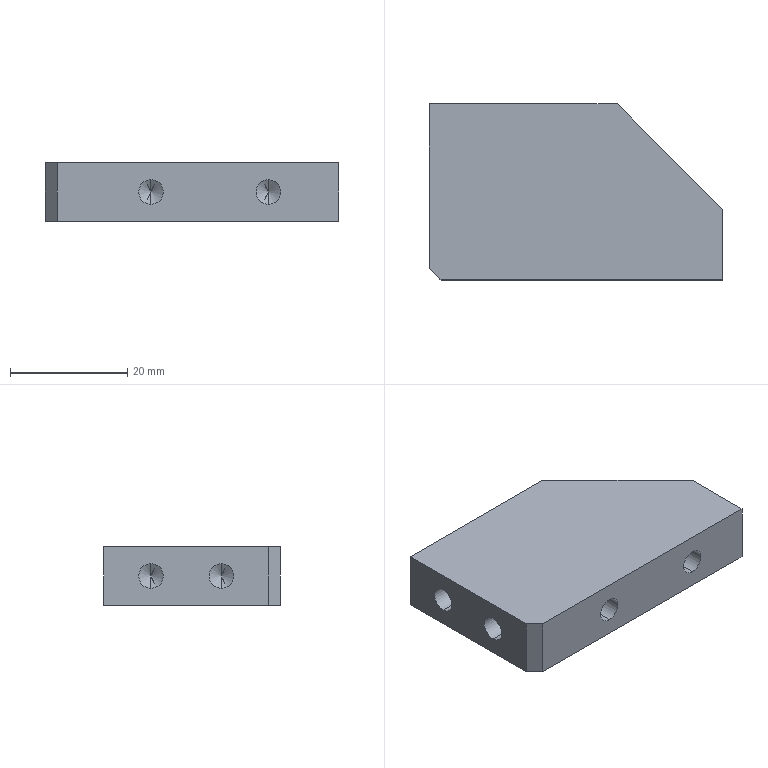Part | SolidWorks | features HoleWzd 2, Chamfer 1, Extrusion 1 | 1 solid | 24 faces | box 50 x 30 x 10 mm | volume 12561 mm3 | cylinder 8 | cone 8 | plane 8 | commonest cylinder face diameters 4.2 x8
STEP:
#1=CARTESIAN_POINT('',(30.,-6.912,7.1));
#2=VERTEX_POINT('',#1);
#3=CARTESIAN_POINT('',(30.,-6.912,2.9));
#4=VERTEX_POINT('',#3);
#5=CARTESIAN_POINT('',(30.,-6.912,5.));
#6=DIRECTION('',(0.,-1.,0.));
#7=DIRECTION('',(0.,0.,-1.));
#8=AXIS2_PLACEMENT_3D('',#5,#6,#7);
#9=CIRCLE('',#8,2.1);
#10=EDGE_CURVE('',#2,#4,#9,.T.);
#11=ORIENTED_EDGE('',*,*,#10,.F.);
#12=CARTESIAN_POINT('',(30.,-20.912,7.1));
#13=VERTEX_POINT('',#12);
#14=CARTESIAN_POINT('',(30.,-20.912,7.1));
#15=DIRECTION('',(0.,-1.,0.));
#16=VECTOR('',#15,1000.);
#17=LINE('',#14,#16);
#18=EDGE_CURVE('',#2,#13,#17,.T.);
#19=ORIENTED_EDGE('',*,*,#18,.T.);
#20=CARTESIAN_POINT('',(30.,-20.912,2.9));
#21=VERTEX_POINT('',#20);
#22=CARTESIAN_POINT('',(30.,-20.912,5.));
#23=DIRECTION('',(0.,-1.,0.));
#24=DIRECTION('',(0.,0.,-1.));
#25=AXIS2_PLACEMENT_3D('',#22,#23,#24);
#26=CIRCLE('',#25,2.1);
#27=EDGE_CURVE('',#13,#21,#26,.T.);
#28=ORIENTED_EDGE('',*,*,#27,.T.);
#29=CARTESIAN_POINT('',(30.,-20.912,2.9));
#30=DIRECTION('',(0.,-1.,0.));
#31=VECTOR('',#30,1000.);
#32=LINE('',#29,#31);
#33=EDGE_CURVE('',#4,#21,#32,.T.);
#34=ORIENTED_EDGE('',*,*,#33,.F.);
#35=EDGE_LOOP('',(#11,#19,#28,#34));
#36=FACE_OUTER_BOUND('',#35,.T.);
#37=CARTESIAN_POINT('',(30.,-20.912,5.));
#38=DIRECTION('',(0.,-1.,0.));
#39=DIRECTION('',(0.,0.,-1.));
#40=AXIS2_PLACEMENT_3D('',#37,#38,#39);
#41=CYLINDRICAL_SURFACE('',#40,2.1);
#42=ADVANCED_FACE('',(#36),#41,.F.);
#43=CARTESIAN_POINT('',(30.,-5.65,5.));
#44=VERTEX_POINT('',#43);
#45=CARTESIAN_POINT('',(30.,-6.912,2.9));
#46=DIRECTION('',(0.,-0.515,-0.8572));
#47=VECTOR('',#46,1000.);
#48=LINE('',#45,#47);
#49=EDGE_CURVE('',#44,#4,#48,.T.);
#50=ORIENTED_EDGE('',*,*,#49,.F.);
#51=CARTESIAN_POINT('',(30.,-6.912,7.1));
#52=DIRECTION('',(0.,-0.515,0.8572));
#53=VECTOR('',#52,1000.);
#54=LINE('',#51,#53);
#55=EDGE_CURVE('',#44,#2,#54,.T.);
#56=ORIENTED_EDGE('',*,*,#55,.T.);
#57=ORIENTED_EDGE('',*,*,#10,.T.);
#58=EDGE_LOOP('',(#50,#56,#57));
#59=FACE_OUTER_BOUND('',#58,.T.);
#60=CARTESIAN_POINT('',(30.,-6.912,5.));
#61=DIRECTION('',(0.,-1.,0.));
#62=DIRECTION('',(0.,0.,-1.));
#63=AXIS2_PLACEMENT_3D('',#60,#61,#62);
#64=CONICAL_SURFACE('',#63,2.1,1.03);
#65=ADVANCED_FACE('',(#59),#64,.F.);
#66=CARTESIAN_POINT('',(50.,-6.912,7.1));
#67=VERTEX_POINT('',#66);
#68=CARTESIAN_POINT('',(50.,-6.912,2.9));
#69=VERTEX_POINT('',#68);
#70=CARTESIAN_POINT('',(50.,-6.912,5.));
#71=DIRECTION('',(0.,-1.,0.));
#72=DIRECTION('',(0.,0.,-1.));
#73=AXIS2_PLACEMENT_3D('',#70,#71,#72);
#74=CIRCLE('',#73,2.1);
#75=EDGE_CURVE('',#67,#69,#74,.T.);
#76=ORIENTED_EDGE('',*,*,#75,.F.);
#77=CARTESIAN_POINT('',(50.,-20.912,7.1));
#78=VERTEX_POINT('',#77);
#79=CARTESIAN_POINT('',(50.,-20.912,7.1));
#80=DIRECTION('',(0.,-1.,0.));
#81=VECTOR('',#80,1000.);
#82=LINE('',#79,#81);
#83=EDGE_CURVE('',#67,#78,#82,.T.);
#84=ORIENTED_EDGE('',*,*,#83,.T.);
#85=CARTESIAN_POINT('',(50.,-20.912,2.9));
#86=VERTEX_POINT('',#85);
#87=CARTESIAN_POINT('',(50.,-20.912,5.));
#88=DIRECTION('',(0.,-1.,0.));
#89=DIRECTION('',(0.,0.,-1.));
#90=AXIS2_PLACEMENT_3D('',#87,#88,#89);
#91=CIRCLE('',#90,2.1);
#92=EDGE_CURVE('',#78,#86,#91,.T.);
#93=ORIENTED_EDGE('',*,*,#92,.T.);
#94=CARTESIAN_POINT('',(50.,-20.912,2.9));
#95=DIRECTION('',(0.,-1.,0.));
#96=VECTOR('',#95,1000.);
#97=LINE('',#94,#96);
#98=EDGE_CURVE('',#69,#86,#97,.T.);
#99=ORIENTED_EDGE('',*,*,#98,.F.);
#100=EDGE_LOOP('',(#76,#84,#93,#99));
#101=FACE_OUTER_BOUND('',#100,.T.);
#102=CARTESIAN_POINT('',(50.,-20.912,5.));
#103=DIRECTION('',(0.,-1.,0.));
#104=DIRECTION('',(0.,0.,-1.));
#105=AXIS2_PLACEMENT_3D('',#102,#103,#104);
#106=CYLINDRICAL_SURFACE('',#105,2.1);
#107=ADVANCED_FACE('',(#101),#106,.F.);
#108=CARTESIAN_POINT('',(50.,-5.65,5.));
#109=VERTEX_POINT('',#108);
#110=CARTESIAN_POINT('',(50.,-6.912,2.9));
#111=DIRECTION('',(0.,-0.515,-0.8572));
#112=VECTOR('',#111,1000.);
#113=LINE('',#110,#112);
#114=EDGE_CURVE('',#109,#69,#113,.T.);
#115=ORIENTED_EDGE('',*,*,#114,.F.);
#116=CARTESIAN_POINT('',(50.,-6.912,7.1));
#117=DIRECTION('',(0.,-0.515,0.8572));
#118=VECTOR('',#117,1000.);
#119=LINE('',#116,#118);
#120=EDGE_CURVE('',#109,#67,#119,.T.);
#121=ORIENTED_EDGE('',*,*,#120,.T.);
#122=ORIENTED_EDGE('',*,*,#75,.T.);
#123=EDGE_LOOP('',(#115,#121,#122));
#124=FACE_OUTER_BOUND('',#123,.T.);
#125=CARTESIAN_POINT('',(50.,-6.912,5.));
#126=DIRECTION('',(0.,-1.,0.));
#127=DIRECTION('',(0.,0.,-1.));
#128=AXIS2_PLACEMENT_3D('',#125,#126,#127);
#129=CONICAL_SURFACE('',#128,2.1,1.03);
#130=ADVANCED_FACE('',(#124),#129,.F.);
#131=CARTESIAN_POINT('',(26.,-10.912,2.9));
#132=VERTEX_POINT('',#131);
#133=CARTESIAN_POINT('',(26.,-10.912,7.1));
#134=VERTEX_POINT('',#133);
#135=CARTESIAN_POINT('',(26.,-10.912,5.));
#136=DIRECTION('',(-1.,0.,0.));
#137=DIRECTION('',(0.,0.,1.));
#138=AXIS2_PLACEMENT_3D('',#135,#136,#137);
#139=CIRCLE('',#138,2.1);
#140=EDGE_CURVE('',#132,#134,#139,.T.);
#141=ORIENTED_EDGE('',*,*,#140,.F.);
#142=CARTESIAN_POINT('',(12.,-10.912,2.9));
#143=VERTEX_POINT('',#142);
#144=CARTESIAN_POINT('',(12.,-10.912,2.9));
#145=DIRECTION('',(-1.,0.,0.));
#146=VECTOR('',#145,1000.);
#147=LINE('',#144,#146);
#148=EDGE_CURVE('',#132,#143,#147,.T.);
#149=ORIENTED_EDGE('',*,*,#148,.T.);
#150=CARTESIAN_POINT('',(12.,-10.912,7.1));
#151=VERTEX_POINT('',#150);
#152=CARTESIAN_POINT('',(12.,-10.912,5.));
#153=DIRECTION('',(-1.,0.,0.));
#154=DIRECTION('',(0.,0.,1.));
#155=AXIS2_PLACEMENT_3D('',#152,#153,#154);
#156=CIRCLE('',#155,2.1);
#157=EDGE_CURVE('',#143,#151,#156,.T.);
#158=ORIENTED_EDGE('',*,*,#157,.T.);
#159=CARTESIAN_POINT('',(12.,-10.912,7.1));
#160=DIRECTION('',(-1.,0.,0.));
#161=VECTOR('',#160,1000.);
#162=LINE('',#159,#161);
#163=EDGE_CURVE('',#134,#151,#162,.T.);
#164=ORIENTED_EDGE('',*,*,#163,.F.);
#165=EDGE_LOOP('',(#141,#149,#158,#164));
#166=FACE_OUTER_BOUND('',#165,.T.);
#167=CARTESIAN_POINT('',(12.,-10.912,5.));
#168=DIRECTION('',(-1.,0.,0.));
#169=DIRECTION('',(0.,0.,1.));
#170=AXIS2_PLACEMENT_3D('',#167,#168,#169);
#171=CYLINDRICAL_SURFACE('',#170,2.1);
#172=ADVANCED_FACE('',(#166),#171,.F.);
#173=CARTESIAN_POINT('',(27.262,-10.912,5.));
#174=VERTEX_POINT('',#173);
#175=CARTESIAN_POINT('',(26.,-10.912,7.1));
#176=DIRECTION('',(-0.515,0.,0.8572));
#177=VECTOR('',#176,1000.);
#178=LINE('',#175,#177);
#179=EDGE_CURVE('',#174,#134,#178,.T.);
#180=ORIENTED_EDGE('',*,*,#179,.F.);
#181=CARTESIAN_POINT('',(26.,-10.912,2.9));
#182=DIRECTION('',(-0.515,0.,-0.8572));
#183=VECTOR('',#182,1000.);
#184=LINE('',#181,#183);
#185=EDGE_CURVE('',#174,#132,#184,.T.);
#186=ORIENTED_EDGE('',*,*,#185,.T.);
#187=ORIENTED_EDGE('',*,*,#140,.T.);
#188=EDGE_LOOP('',(#180,#186,#187));
#189=FACE_OUTER_BOUND('',#188,.T.);
#190=CARTESIAN_POINT('',(26.,-10.912,5.));
#191=DIRECTION('',(-1.,0.,0.));
#192=DIRECTION('',(0.,0.,1.));
#193=AXIS2_PLACEMENT_3D('',#190,#191,#192);
#194=CONICAL_SURFACE('',#193,2.1,1.03);
#195=ADVANCED_FACE('',(#189),#194,.F.);
#196=CARTESIAN_POINT('',(26.,1.088,2.9));
#197=VERTEX_POINT('',#196);
#198=CARTESIAN_POINT('',(26.,1.088,7.1));
#199=VERTEX_POINT('',#198);
#200=CARTESIAN_POINT('',(26.,1.088,5.));
#201=DIRECTION('',(-1.,0.,0.));
#202=DIRECTION('',(0.,0.,1.));
#203=AXIS2_PLACEMENT_3D('',#200,#201,#202);
#204=CIRCLE('',#203,2.1);
#205=EDGE_CURVE('',#197,#199,#204,.T.);
#206=ORIENTED_EDGE('',*,*,#205,.F.);
#207=CARTESIAN_POINT('',(12.,1.088,2.9));
#208=VERTEX_POINT('',#207);
#209=CARTESIAN_POINT('',(12.,1.088,2.9));
#210=DIRECTION('',(-1.,0.,0.));
#211=VECTOR('',#210,1000.);
#212=LINE('',#209,#211);
#213=EDGE_CURVE('',#197,#208,#212,.T.);
#214=ORIENTED_EDGE('',*,*,#213,.T.);
#215=CARTESIAN_POINT('',(12.,1.088,7.1));
#216=VERTEX_POINT('',#215);
#217=CARTESIAN_POINT('',(12.,1.088,5.));
#218=DIRECTION('',(-1.,0.,0.));
#219=DIRECTION('',(0.,0.,1.));
#220=AXIS2_PLACEMENT_3D('',#217,#218,#219);
#221=CIRCLE('',#220,2.1);
#222=EDGE_CURVE('',#208,#216,#221,.T.);
#223=ORIENTED_EDGE('',*,*,#222,.T.);
#224=CARTESIAN_POINT('',(12.,1.088,7.1));
#225=DIRECTION('',(-1.,0.,0.));
#226=VECTOR('',#225,1000.);
#227=LINE('',#224,#226);
#228=EDGE_CURVE('',#199,#216,#227,.T.);
#229=ORIENTED_EDGE('',*,*,#228,.F.);
#230=EDGE_LOOP('',(#206,#214,#223,#229));
#231=FACE_OUTER_BOUND('',#230,.T.);
#232=CARTESIAN_POINT('',(12.,1.088,5.));
#233=DIRECTION('',(-1.,0.,0.));
#234=DIRECTION('',(0.,0.,1.));
#235=AXIS2_PLACEMENT_3D('',#232,#233,#234);
#236=CYLINDRICAL_SURFACE('',#235,2.1);
#237=ADVANCED_FACE('',(#231),#236,.F.);
#238=CARTESIAN_POINT('',(27.262,1.088,5.));
#239=VERTEX_POINT('',#238);
#240=CARTESIAN_POINT('',(26.,1.088,7.1));
#241=DIRECTION('',(-0.515,0.,0.8572));
#242=VECTOR('',#241,1000.);
#243=LINE('',#240,#242);
#244=EDGE_CURVE('',#239,#199,#243,.T.);
#245=ORIENTED_EDGE('',*,*,#244,.F.);
#246=CARTESIAN_POINT('',(26.,1.088,2.9));
#247=DIRECTION('',(-0.515,0.,-0.8572));
#248=VECTOR('',#247,1000.);
#249=LINE('',#246,#248);
#250=EDGE_CURVE('',#239,#197,#249,.T.);
#251=ORIENTED_EDGE('',*,*,#250,.T.);
#252=ORIENTED_EDGE('',*,*,#205,.T.);
#253=EDGE_LOOP('',(#245,#251,#252));
#254=FACE_OUTER_BOUND('',#253,.T.);
#255=CARTESIAN_POINT('',(26.,1.088,5.));
#256=DIRECTION('',(-1.,0.,0.));
#257=DIRECTION('',(0.,0.,1.));
#258=AXIS2_PLACEMENT_3D('',#255,#256,#257);
#259=CONICAL_SURFACE('',#258,2.1,1.03);
#260=ADVANCED_FACE('',(#254),#259,.F.);
#261=CARTESIAN_POINT('',(62.,-20.912,0.));
#262=VERTEX_POINT('',#261);
#263=CARTESIAN_POINT('',(62.,-8.912,0.));
#264=VERTEX_POINT('',#263);
#265=CARTESIAN_POINT('',(62.,-8.912,0.));
#266=DIRECTION('',(0.,1.,0.));
#267=VECTOR('',#266,1000.);
#268=LINE('',#265,#267);
#269=EDGE_CURVE('',#262,#264,#268,.T.);
#270=ORIENTED_EDGE('',*,*,#269,.T.);
#271=CARTESIAN_POINT('',(62.,-8.912,10.));
#272=VERTEX_POINT('',#271);
#273=CARTESIAN_POINT('',(62.,-8.912,10.));
#274=DIRECTION('',(0.,0.,-1.));
#275=VECTOR('',#274,1000.);
#276=LINE('',#273,#275);
#277=EDGE_CURVE('',#272,#264,#276,.T.);
#278=ORIENTED_EDGE('',*,*,#277,.F.);
#279=CARTESIAN_POINT('',(62.,-20.912,10.));
#280=VERTEX_POINT('',#279);
#281=CARTESIAN_POINT('',(62.,-8.912,10.));
#282=DIRECTION('',(0.,1.,0.));
#283=VECTOR('',#282,1000.);
#284=LINE('',#281,#283);
#285=EDGE_CURVE('',#280,#272,#284,.T.);
#286=ORIENTED_EDGE('',*,*,#285,.F.);
#287=CARTESIAN_POINT('',(62.,-20.912,10.));
#288=DIRECTION('',(0.,0.,-1.));
#289=VECTOR('',#288,1000.);
#290=LINE('',#287,#289);
#291=EDGE_CURVE('',#280,#262,#290,.T.);
#292=ORIENTED_EDGE('',*,*,#291,.T.);
#293=EDGE_LOOP('',(#270,#278,#286,#292));
#294=FACE_OUTER_BOUND('',#293,.T.);
#295=CARTESIAN_POINT('',(62.,-8.912,10.));
#296=DIRECTION('',(-1.,0.,0.));
#297=DIRECTION('',(0.,0.,1.));
#298=AXIS2_PLACEMENT_3D('',#295,#296,#297);
#299=PLANE('',#298);
#300=ADVANCED_FACE('',(#294),#299,.F.);
#301=CARTESIAN_POINT('',(44.,9.088,0.));
#302=VERTEX_POINT('',#301);
#303=CARTESIAN_POINT('',(44.,9.088,0.));
#304=DIRECTION('',(-0.7071,0.7071,0.));
#305=VECTOR('',#304,1000.);
#306=LINE('',#303,#305);
#307=EDGE_CURVE('',#264,#302,#306,.T.);
#308=ORIENTED_EDGE('',*,*,#307,.T.);
#309=CARTESIAN_POINT('',(44.,9.088,10.));
#310=VERTEX_POINT('',#309);
#311=CARTESIAN_POINT('',(44.,9.088,10.));
#312=DIRECTION('',(0.,0.,-1.));
#313=VECTOR('',#312,1000.);
#314=LINE('',#311,#313);
#315=EDGE_CURVE('',#310,#302,#314,.T.);
#316=ORIENTED_EDGE('',*,*,#315,.F.);
#317=CARTESIAN_POINT('',(44.,9.088,10.));
#318=DIRECTION('',(-0.7071,0.7071,0.));
#319=VECTOR('',#318,1000.);
#320=LINE('',#317,#319);
#321=EDGE_CURVE('',#272,#310,#320,.T.);
#322=ORIENTED_EDGE('',*,*,#321,.F.);
#323=ORIENTED_EDGE('',*,*,#277,.T.);
#324=EDGE_LOOP('',(#308,#316,#322,#323));
#325=FACE_OUTER_BOUND('',#324,.T.);
#326=CARTESIAN_POINT('',(44.,9.088,10.));
#327=DIRECTION('',(-0.7071,-0.7071,0.));
#328=DIRECTION('',(0.7071,-0.7071,0.));
#329=AXIS2_PLACEMENT_3D('',#326,#327,#328);
#330=PLANE('',#329);
#331=ADVANCED_FACE('',(#325),#330,.F.);
#332=CARTESIAN_POINT('',(12.,9.088,0.));
#333=VERTEX_POINT('',#332);
#334=CARTESIAN_POINT('',(12.,9.088,0.));
#335=DIRECTION('',(-1.,0.,0.));
#336=VECTOR('',#335,1000.);
#337=LINE('',#334,#336);
#338=EDGE_CURVE('',#302,#333,#337,.T.);
#339=ORIENTED_EDGE('',*,*,#338,.T.);
#340=CARTESIAN_POINT('',(12.,9.088,10.));
#341=VERTEX_POINT('',#340);
#342=CARTESIAN_POINT('',(12.,9.088,10.));
#343=DIRECTION('',(0.,0.,-1.));
#344=VECTOR('',#343,1000.);
#345=LINE('',#342,#344);
#346=EDGE_CURVE('',#341,#333,#345,.T.);
#347=ORIENTED_EDGE('',*,*,#346,.F.);
#348=CARTESIAN_POINT('',(12.,9.088,10.));
#349=DIRECTION('',(-1.,0.,0.));
#350=VECTOR('',#349,1000.);
#351=LINE('',#348,#350);
#352=EDGE_CURVE('',#310,#341,#351,.T.);
#353=ORIENTED_EDGE('',*,*,#352,.F.);
#354=ORIENTED_EDGE('',*,*,#315,.T.);
#355=EDGE_LOOP('',(#339,#347,#353,#354));
#356=FACE_OUTER_BOUND('',#355,.T.);
#357=CARTESIAN_POINT('',(12.,9.088,10.));
#358=DIRECTION('',(0.,-1.,0.));
#359=DIRECTION('',(0.,0.,-1.));
#360=AXIS2_PLACEMENT_3D('',#357,#358,#359);
#361=PLANE('',#360);
#362=ADVANCED_FACE('',(#356),#361,.F.);
#363=CARTESIAN_POINT('',(12.,-10.912,5.));
#364=DIRECTION('',(-1.,0.,0.));
#365=DIRECTION('',(0.,0.,1.));
#366=AXIS2_PLACEMENT_3D('',#363,#364,#365);
#367=CIRCLE('',#366,2.1);
#368=EDGE_CURVE('',#151,#143,#367,.T.);
#369=ORIENTED_EDGE('',*,*,#368,.F.);
#370=ORIENTED_EDGE('',*,*,#157,.F.);
#371=EDGE_LOOP('',(#369,#370));
#372=FACE_BOUND('',#371,.T.);
#373=CARTESIAN_POINT('',(12.,1.088,5.));
#374=DIRECTION('',(-1.,0.,0.));
#375=DIRECTION('',(0.,0.,1.));
#376=AXIS2_PLACEMENT_3D('',#373,#374,#375);
#377=CIRCLE('',#376,2.1);
#378=EDGE_CURVE('',#216,#208,#377,.T.);
#379=ORIENTED_EDGE('',*,*,#378,.F.);
#380=ORIENTED_EDGE('',*,*,#222,.F.);
#381=EDGE_LOOP('',(#379,#380));
#382=FACE_BOUND('',#381,.T.);
#383=CARTESIAN_POINT('',(12.,-18.912,0.));
#384=VERTEX_POINT('',#383);
#385=CARTESIAN_POINT('',(12.,-20.912,0.));
#386=DIRECTION('',(0.,-1.,0.));
#387=VECTOR('',#386,1000.);
#388=LINE('',#385,#387);
#389=EDGE_CURVE('',#333,#384,#388,.T.);
#390=ORIENTED_EDGE('',*,*,#389,.T.);
#391=CARTESIAN_POINT('',(12.,-18.912,10.));
#392=VERTEX_POINT('',#391);
#393=CARTESIAN_POINT('',(12.,-18.912,10.));
#394=DIRECTION('',(0.,0.,1.));
#395=VECTOR('',#394,1000.);
#396=LINE('',#393,#395);
#397=EDGE_CURVE('',#384,#392,#396,.T.);
#398=ORIENTED_EDGE('',*,*,#397,.T.);
#399=CARTESIAN_POINT('',(12.,-20.912,10.));
#400=DIRECTION('',(0.,-1.,0.));
#401=VECTOR('',#400,1000.);
#402=LINE('',#399,#401);
#403=EDGE_CURVE('',#341,#392,#402,.T.);
#404=ORIENTED_EDGE('',*,*,#403,.F.);
#405=ORIENTED_EDGE('',*,*,#346,.T.);
#406=EDGE_LOOP('',(#390,#398,#404,#405));
#407=FACE_OUTER_BOUND('',#406,.T.);
#408=CARTESIAN_POINT('',(12.,-20.912,10.));
#409=DIRECTION('',(1.,0.,0.));
#410=DIRECTION('',(0.,1.,0.));
#411=AXIS2_PLACEMENT_3D('',#408,#409,#410);
#412=PLANE('',#411);
#413=ADVANCED_FACE('',(#372,#382,#407),#412,.F.);
#414=CARTESIAN_POINT('',(30.,-20.912,5.));
#415=DIRECTION('',(0.,-1.,0.));
#416=DIRECTION('',(0.,0.,-1.));
#417=AXIS2_PLACEMENT_3D('',#414,#415,#416);
#418=CIRCLE('',#417,2.1);
#419=EDGE_CURVE('',#21,#13,#418,.T.);
#420=ORIENTED_EDGE('',*,*,#419,.F.);
#421=ORIENTED_EDGE('',*,*,#27,.F.);
#422=EDGE_LOOP('',(#420,#421));
#423=FACE_BOUND('',#422,.T.);
#424=CARTESIAN_POINT('',(50.,-20.912,5.));
#425=DIRECTION('',(0.,-1.,0.));
#426=DIRECTION('',(0.,0.,-1.));
#427=AXIS2_PLACEMENT_3D('',#424,#425,#426);
#428=CIRCLE('',#427,2.1);
#429=EDGE_CURVE('',#86,#78,#428,.T.);
#430=ORIENTED_EDGE('',*,*,#429,.F.);
#431=ORIENTED_EDGE('',*,*,#92,.F.);
#432=EDGE_LOOP('',(#430,#431));
#433=FACE_BOUND('',#432,.T.);
#434=CARTESIAN_POINT('',(14.,-20.912,10.));
#435=VERTEX_POINT('',#434);
#436=CARTESIAN_POINT('',(62.,-20.912,10.));
#437=DIRECTION('',(1.,0.,0.));
#438=VECTOR('',#437,1000.);
#439=LINE('',#436,#438);
#440=EDGE_CURVE('',#435,#280,#439,.T.);
#441=ORIENTED_EDGE('',*,*,#440,.F.);
#442=CARTESIAN_POINT('',(14.,-20.912,0.));
#443=VERTEX_POINT('',#442);
#444=CARTESIAN_POINT('',(14.,-20.912,10.));
#445=DIRECTION('',(0.,0.,-1.));
#446=VECTOR('',#445,1000.);
#447=LINE('',#444,#446);
#448=EDGE_CURVE('',#435,#443,#447,.T.);
#449=ORIENTED_EDGE('',*,*,#448,.T.);
#450=CARTESIAN_POINT('',(62.,-20.912,0.));
#451=DIRECTION('',(1.,0.,0.));
#452=VECTOR('',#451,1000.);
#453=LINE('',#450,#452);
#454=EDGE_CURVE('',#443,#262,#453,.T.);
#455=ORIENTED_EDGE('',*,*,#454,.T.);
#456=ORIENTED_EDGE('',*,*,#291,.F.);
#457=EDGE_LOOP('',(#441,#449,#455,#456));
#458=FACE_OUTER_BOUND('',#457,.T.);
#459=CARTESIAN_POINT('',(62.,-20.912,10.));
#460=DIRECTION('',(0.,1.,0.));
#461=DIRECTION('',(-1.,0.,0.));
#462=AXIS2_PLACEMENT_3D('',#459,#460,#461);
#463=PLANE('',#462);
#464=ADVANCED_FACE('',(#423,#433,#458),#463,.F.);
#465=ORIENTED_EDGE('',*,*,#403,.T.);
#466=CARTESIAN_POINT('',(14.,-20.912,10.));
#467=DIRECTION('',(0.7071,-0.7071,0.));
#468=VECTOR('',#467,1000.);
#469=LINE('',#466,#468);
#470=EDGE_CURVE('',#392,#435,#469,.T.);
#471=ORIENTED_EDGE('',*,*,#470,.T.);
#472=ORIENTED_EDGE('',*,*,#440,.T.);
#473=ORIENTED_EDGE('',*,*,#285,.T.);
#474=ORIENTED_EDGE('',*,*,#321,.T.);
#475=ORIENTED_EDGE('',*,*,#352,.T.);
#476=EDGE_LOOP('',(#465,#471,#472,#473,#474,#475));
#477=FACE_OUTER_BOUND('',#476,.T.);
#478=CARTESIAN_POINT('',(0.,0.,10.));
#479=DIRECTION('',(0.,0.,-1.));
#480=DIRECTION('',(-1.,0.,0.));
#481=AXIS2_PLACEMENT_3D('',#478,#479,#480);
#482=PLANE('',#481);
#483=ADVANCED_FACE('',(#477),#482,.F.);
#484=ORIENTED_EDGE('',*,*,#454,.F.);
#485=CARTESIAN_POINT('',(-3.456,-3.456,0.));
#486=DIRECTION('',(-0.7071,0.7071,0.));
#487=VECTOR('',#486,1000.);
#488=LINE('',#485,#487);
#489=EDGE_CURVE('',#443,#384,#488,.T.);
#490=ORIENTED_EDGE('',*,*,#489,.T.);
#491=ORIENTED_EDGE('',*,*,#389,.F.);
#492=ORIENTED_EDGE('',*,*,#338,.F.);
#493=ORIENTED_EDGE('',*,*,#307,.F.);
#494=ORIENTED_EDGE('',*,*,#269,.F.);
#495=EDGE_LOOP('',(#484,#490,#491,#492,#493,#494));
#496=FACE_OUTER_BOUND('',#495,.T.);
#497=CARTESIAN_POINT('',(0.,0.,0.));
#498=DIRECTION('',(0.,0.,-1.));
#499=DIRECTION('',(-1.,0.,0.));
#500=AXIS2_PLACEMENT_3D('',#497,#498,#499);
#501=PLANE('',#500);
#502=ADVANCED_FACE('',(#496),#501,.T.);
#503=ORIENTED_EDGE('',*,*,#470,.F.);
#504=ORIENTED_EDGE('',*,*,#397,.F.);
#505=ORIENTED_EDGE('',*,*,#489,.F.);
#506=ORIENTED_EDGE('',*,*,#448,.F.);
#507=EDGE_LOOP('',(#503,#504,#505,#506));
#508=FACE_OUTER_BOUND('',#507,.T.);
#509=CARTESIAN_POINT('',(14.,-20.912,10.));
#510=DIRECTION('',(0.7071,0.7071,0.));
#511=DIRECTION('',(0.,0.,-1.));
#512=AXIS2_PLACEMENT_3D('',#509,#510,#511);
#513=PLANE('',#512);
#514=ADVANCED_FACE('',(#508),#513,.F.);
#515=ORIENTED_EDGE('',*,*,#250,.F.);
#516=ORIENTED_EDGE('',*,*,#244,.T.);
#517=CARTESIAN_POINT('',(26.,1.088,5.));
#518=DIRECTION('',(-1.,0.,0.));
#519=DIRECTION('',(0.,0.,1.));
#520=AXIS2_PLACEMENT_3D('',#517,#518,#519);
#521=CIRCLE('',#520,2.1);
#522=EDGE_CURVE('',#199,#197,#521,.T.);
#523=ORIENTED_EDGE('',*,*,#522,.T.);
#524=EDGE_LOOP('',(#515,#516,#523));
#525=FACE_OUTER_BOUND('',#524,.T.);
#526=CARTESIAN_POINT('',(26.,1.088,5.));
#527=DIRECTION('',(-1.,0.,0.));
#528=DIRECTION('',(0.,0.,1.));
#529=AXIS2_PLACEMENT_3D('',#526,#527,#528);
#530=CONICAL_SURFACE('',#529,2.1,1.03);
#531=ADVANCED_FACE('',(#525),#530,.F.);
#532=ORIENTED_EDGE('',*,*,#213,.F.);
#533=ORIENTED_EDGE('',*,*,#522,.F.);
#534=ORIENTED_EDGE('',*,*,#228,.T.);
#535=ORIENTED_EDGE('',*,*,#378,.T.);
#536=EDGE_LOOP('',(#532,#533,#534,#535));
#537=FACE_OUTER_BOUND('',#536,.T.);
#538=CARTESIAN_POINT('',(12.,1.088,5.));
#539=DIRECTION('',(-1.,0.,0.));
#540=DIRECTION('',(0.,0.,1.));
#541=AXIS2_PLACEMENT_3D('',#538,#539,#540);
#542=CYLINDRICAL_SURFACE('',#541,2.1);
#543=ADVANCED_FACE('',(#537),#542,.F.);
#544=ORIENTED_EDGE('',*,*,#185,.F.);
#545=ORIENTED_EDGE('',*,*,#179,.T.);
#546=CARTESIAN_POINT('',(26.,-10.912,5.));
#547=DIRECTION('',(-1.,0.,0.));
#548=DIRECTION('',(0.,0.,1.));
#549=AXIS2_PLACEMENT_3D('',#546,#547,#548);
#550=CIRCLE('',#549,2.1);
#551=EDGE_CURVE('',#134,#132,#550,.T.);
#552=ORIENTED_EDGE('',*,*,#551,.T.);
#553=EDGE_LOOP('',(#544,#545,#552));
#554=FACE_OUTER_BOUND('',#553,.T.);
#555=CARTESIAN_POINT('',(26.,-10.912,5.));
#556=DIRECTION('',(-1.,0.,0.));
#557=DIRECTION('',(0.,0.,1.));
#558=AXIS2_PLACEMENT_3D('',#555,#556,#557);
#559=CONICAL_SURFACE('',#558,2.1,1.03);
#560=ADVANCED_FACE('',(#554),#559,.F.);
#561=ORIENTED_EDGE('',*,*,#148,.F.);
#562=ORIENTED_EDGE('',*,*,#551,.F.);
#563=ORIENTED_EDGE('',*,*,#163,.T.);
#564=ORIENTED_EDGE('',*,*,#368,.T.);
#565=EDGE_LOOP('',(#561,#562,#563,#564));
#566=FACE_OUTER_BOUND('',#565,.T.);
#567=CARTESIAN_POINT('',(12.,-10.912,5.));
#568=DIRECTION('',(-1.,0.,0.));
#569=DIRECTION('',(0.,0.,1.));
#570=AXIS2_PLACEMENT_3D('',#567,#568,#569);
#571=CYLINDRICAL_SURFACE('',#570,2.1);
#572=ADVANCED_FACE('',(#566),#571,.F.);
#573=ORIENTED_EDGE('',*,*,#120,.F.);
#574=ORIENTED_EDGE('',*,*,#114,.T.);
#575=CARTESIAN_POINT('',(50.,-6.912,5.));
#576=DIRECTION('',(0.,-1.,0.));
#577=DIRECTION('',(0.,0.,-1.));
#578=AXIS2_PLACEMENT_3D('',#575,#576,#577);
#579=CIRCLE('',#578,2.1);
#580=EDGE_CURVE('',#69,#67,#579,.T.);
#581=ORIENTED_EDGE('',*,*,#580,.T.);
#582=EDGE_LOOP('',(#573,#574,#581));
#583=FACE_OUTER_BOUND('',#582,.T.);
#584=CARTESIAN_POINT('',(50.,-6.912,5.));
#585=DIRECTION('',(0.,-1.,0.));
#586=DIRECTION('',(0.,0.,-1.));
#587=AXIS2_PLACEMENT_3D('',#584,#585,#586);
#588=CONICAL_SURFACE('',#587,2.1,1.03);
#589=ADVANCED_FACE('',(#583),#588,.F.);
#590=ORIENTED_EDGE('',*,*,#83,.F.);
#591=ORIENTED_EDGE('',*,*,#580,.F.);
#592=ORIENTED_EDGE('',*,*,#98,.T.);
#593=ORIENTED_EDGE('',*,*,#429,.T.);
#594=EDGE_LOOP('',(#590,#591,#592,#593));
#595=FACE_OUTER_BOUND('',#594,.T.);
#596=CARTESIAN_POINT('',(50.,-20.912,5.));
#597=DIRECTION('',(0.,-1.,0.));
#598=DIRECTION('',(0.,0.,-1.));
#599=AXIS2_PLACEMENT_3D('',#596,#597,#598);
#600=CYLINDRICAL_SURFACE('',#599,2.1);
#601=ADVANCED_FACE('',(#595),#600,.F.);
#602=ORIENTED_EDGE('',*,*,#55,.F.);
#603=ORIENTED_EDGE('',*,*,#49,.T.);
#604=CARTESIAN_POINT('',(30.,-6.912,5.));
#605=DIRECTION('',(0.,-1.,0.));
#606=DIRECTION('',(0.,0.,-1.));
#607=AXIS2_PLACEMENT_3D('',#604,#605,#606);
#608=CIRCLE('',#607,2.1);
#609=EDGE_CURVE('',#4,#2,#608,.T.);
#610=ORIENTED_EDGE('',*,*,#609,.T.);
#611=EDGE_LOOP('',(#602,#603,#610));
#612=FACE_OUTER_BOUND('',#611,.T.);
#613=CARTESIAN_POINT('',(30.,-6.912,5.));
#614=DIRECTION('',(0.,-1.,0.));
#615=DIRECTION('',(0.,0.,-1.));
#616=AXIS2_PLACEMENT_3D('',#613,#614,#615);
#617=CONICAL_SURFACE('',#616,2.1,1.03);
#618=ADVANCED_FACE('',(#612),#617,.F.);
#619=ORIENTED_EDGE('',*,*,#18,.F.);
#620=ORIENTED_EDGE('',*,*,#609,.F.);
#621=ORIENTED_EDGE('',*,*,#33,.T.);
#622=ORIENTED_EDGE('',*,*,#419,.T.);
#623=EDGE_LOOP('',(#619,#620,#621,#622));
#624=FACE_OUTER_BOUND('',#623,.T.);
#625=CARTESIAN_POINT('',(30.,-20.912,5.));
#626=DIRECTION('',(0.,-1.,0.));
#627=DIRECTION('',(0.,0.,-1.));
#628=AXIS2_PLACEMENT_3D('',#625,#626,#627);
#629=CYLINDRICAL_SURFACE('',#628,2.1);
#630=ADVANCED_FACE('',(#624),#629,.F.);
#631=CLOSED_SHELL('',(#42,#65,#107,#130,#172,#195,#237,#260,#300,#331,#362,#413,#464,#483,#502,#514,#531,#543,#560,#572,#589,#601,#618,#630));
#632=MANIFOLD_SOLID_BREP('',#631);
#633=CARTESIAN_POINT('',(0.,0.,0.));
#634=DIRECTION('',(0.,0.,1.));
#635=DIRECTION('',(1.,0.,0.));
#636=AXIS2_PLACEMENT_3D('',#633,#634,#635);
#637=(LENGTH_UNIT()NAMED_UNIT(*)SI_UNIT(.MILLI.,.METRE.));
#638=UNCERTAINTY_MEASURE_WITH_UNIT(LENGTH_MEASURE(0.00001),#637,'','');
#639=(NAMED_UNIT(*)PLANE_ANGLE_UNIT()SI_UNIT($,.RADIAN.));
#640=(NAMED_UNIT(*)SI_UNIT($,.STERADIAN.)SOLID_ANGLE_UNIT());
#641=(GEOMETRIC_REPRESENTATION_CONTEXT(3)GLOBAL_UNCERTAINTY_ASSIGNED_CONTEXT((#638))GLOBAL_UNIT_ASSIGNED_CONTEXT((#637,#639,#640))REPRESENTATION_CONTEXT('',''));
#642=ADVANCED_BREP_SHAPE_REPRESENTATION('',(#632,#636),#641);